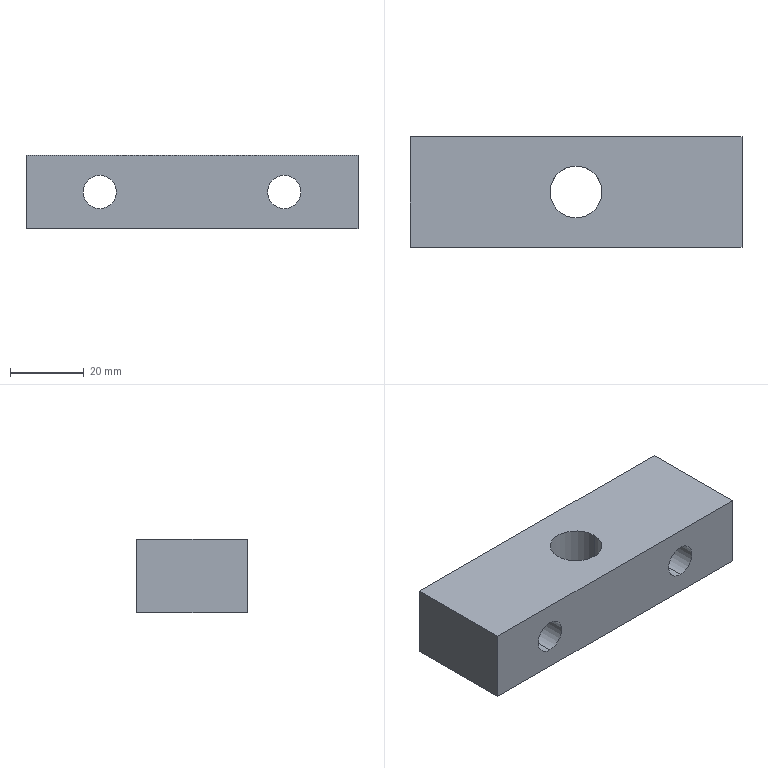Part | STEP file | M-05-2507_default | 1 solid | 18 faces | box 90 x 30 x 20 mm | volume 45159 mm3 | cylinder 10 | plane 8 | commonest cylinder face diameters 9 x4 15 x4 14 x2
STEP:
#1=CARTESIAN_POINT('',(0.,0.,0.));
#2=DIRECTION('',(0.,0.,1.));
#3=DIRECTION('',(1.,0.,0.));
#4=AXIS2_PLACEMENT_3D('',#1,#2,#3);
#5=CARTESIAN_POINT('',(38.,15.,20.));
#6=VERTEX_POINT('',#5);
#7=CARTESIAN_POINT('',(38.,15.,0.));
#8=VERTEX_POINT('',#7);
#9=CARTESIAN_POINT('',(38.,15.,0.));
#10=DIRECTION('',(0.,0.,-1.));
#11=VECTOR('',#10,1.);
#12=LINE('',#9,#11);
#13=CARTESIAN_POINT('',(45.,15.,0.));
#14=DIRECTION('',(0.,0.,-1.));
#15=DIRECTION('',(-1.,0.,0.));
#16=AXIS2_PLACEMENT_3D('',#13,#14,#15);
#17=CYLINDRICAL_SURFACE('',#16,7.);
#18=CARTESIAN_POINT('',(6.283,0.));
#19=DIRECTION('',(0.,1.));
#20=VECTOR('',#19,1.);
#21=LINE('',#18,#20);
#22=(GEOMETRIC_REPRESENTATION_CONTEXT(2)PARAMETRIC_REPRESENTATION_CONTEXT()REPRESENTATION_CONTEXT('',''));
#23=DEFINITIONAL_REPRESENTATION('',(#21),#22);
#24=PCURVE('',#17,#23);
#25=CARTESIAN_POINT('',(45.,15.,0.));
#26=DIRECTION('',(0.,0.,-1.));
#27=DIRECTION('',(-1.,0.,0.));
#28=AXIS2_PLACEMENT_3D('',#25,#26,#27);
#29=CYLINDRICAL_SURFACE('',#28,7.);
#30=CARTESIAN_POINT('',(0.,0.));
#31=DIRECTION('',(0.,1.));
#32=VECTOR('',#31,1.);
#33=LINE('',#30,#32);
#34=(GEOMETRIC_REPRESENTATION_CONTEXT(2)PARAMETRIC_REPRESENTATION_CONTEXT()REPRESENTATION_CONTEXT('',''));
#35=DEFINITIONAL_REPRESENTATION('',(#33),#34);
#36=PCURVE('',#29,#35);
#37=SURFACE_CURVE('',#12,(#24,#36),.PCURVE_S1.);
#38=EDGE_CURVE('',#6,#8,#37,.T.);
#39=ORIENTED_EDGE('',*,*,#38,.T.);
#40=CARTESIAN_POINT('',(52.,15.,0.));
#41=VERTEX_POINT('',#40);
#42=CARTESIAN_POINT('',(45.,15.,0.));
#43=DIRECTION('',(0.,0.,-1.));
#44=DIRECTION('',(-1.,0.,0.));
#45=AXIS2_PLACEMENT_3D('',#42,#43,#44);
#46=CIRCLE('',#45,7.);
#47=CARTESIAN_POINT('',(0.,0.));
#48=DIRECTION('',(1.,0.));
#49=VECTOR('',#48,1.);
#50=LINE('',#47,#49);
#51=(GEOMETRIC_REPRESENTATION_CONTEXT(2)PARAMETRIC_REPRESENTATION_CONTEXT()REPRESENTATION_CONTEXT('',''));
#52=DEFINITIONAL_REPRESENTATION('',(#50),#51);
#53=PCURVE('',#17,#52);
#54=CARTESIAN_POINT('',(0.,30.,0.));
#55=DIRECTION('',(0.,0.,-1.));
#56=DIRECTION('',(-1.,0.,0.));
#57=AXIS2_PLACEMENT_3D('',#54,#55,#56);
#58=PLANE('',#57);
#59=CARTESIAN_POINT('',(-45.,-15.));
#60=DIRECTION('',(1.,0.));
#61=AXIS2_PLACEMENT_2D('',#59,#60);
#62=CIRCLE('',#61,7.);
#63=(GEOMETRIC_REPRESENTATION_CONTEXT(2)PARAMETRIC_REPRESENTATION_CONTEXT()REPRESENTATION_CONTEXT('',''));
#64=DEFINITIONAL_REPRESENTATION('',(#62),#63);
#65=PCURVE('',#58,#64);
#66=SURFACE_CURVE('',#46,(#53,#65),.PCURVE_S1.);
#67=EDGE_CURVE('',#41,#8,#66,.T.);
#68=ORIENTED_EDGE('',*,*,#67,.F.);
#69=CARTESIAN_POINT('',(52.,15.,20.));
#70=VERTEX_POINT('',#69);
#71=CARTESIAN_POINT('',(52.,15.,0.));
#72=DIRECTION('',(0.,0.,-1.));
#73=VECTOR('',#72,1.);
#74=LINE('',#71,#73);
#75=CARTESIAN_POINT('',(3.142,0.));
#76=DIRECTION('',(0.,1.));
#77=VECTOR('',#76,1.);
#78=LINE('',#75,#77);
#79=(GEOMETRIC_REPRESENTATION_CONTEXT(2)PARAMETRIC_REPRESENTATION_CONTEXT()REPRESENTATION_CONTEXT('',''));
#80=DEFINITIONAL_REPRESENTATION('',(#78),#79);
#81=PCURVE('',#17,#80);
#82=CARTESIAN_POINT('',(3.142,0.));
#83=DIRECTION('',(0.,1.));
#84=VECTOR('',#83,1.);
#85=LINE('',#82,#84);
#86=(GEOMETRIC_REPRESENTATION_CONTEXT(2)PARAMETRIC_REPRESENTATION_CONTEXT()REPRESENTATION_CONTEXT('',''));
#87=DEFINITIONAL_REPRESENTATION('',(#85),#86);
#88=PCURVE('',#29,#87);
#89=SURFACE_CURVE('',#74,(#81,#88),.PCURVE_S1.);
#90=EDGE_CURVE('',#70,#41,#89,.T.);
#91=ORIENTED_EDGE('',*,*,#90,.F.);
#92=CARTESIAN_POINT('',(45.,15.,20.));
#93=DIRECTION('',(0.,0.,-1.));
#94=DIRECTION('',(-1.,0.,0.));
#95=AXIS2_PLACEMENT_3D('',#92,#93,#94);
#96=CIRCLE('',#95,7.);
#97=CARTESIAN_POINT('',(0.,-20.));
#98=DIRECTION('',(1.,0.));
#99=VECTOR('',#98,1.);
#100=LINE('',#97,#99);
#101=(GEOMETRIC_REPRESENTATION_CONTEXT(2)PARAMETRIC_REPRESENTATION_CONTEXT()REPRESENTATION_CONTEXT('',''));
#102=DEFINITIONAL_REPRESENTATION('',(#100),#101);
#103=PCURVE('',#17,#102);
#104=CARTESIAN_POINT('',(0.,30.,20.));
#105=DIRECTION('',(0.,0.,-1.));
#106=DIRECTION('',(-1.,0.,0.));
#107=AXIS2_PLACEMENT_3D('',#104,#105,#106);
#108=PLANE('',#107);
#109=CARTESIAN_POINT('',(-45.,-15.));
#110=DIRECTION('',(1.,0.));
#111=AXIS2_PLACEMENT_2D('',#109,#110);
#112=CIRCLE('',#111,7.);
#113=(GEOMETRIC_REPRESENTATION_CONTEXT(2)PARAMETRIC_REPRESENTATION_CONTEXT()REPRESENTATION_CONTEXT('',''));
#114=DEFINITIONAL_REPRESENTATION('',(#112),#113);
#115=PCURVE('',#108,#114);
#116=SURFACE_CURVE('',#96,(#103,#115),.PCURVE_S1.);
#117=EDGE_CURVE('',#70,#6,#116,.T.);
#118=ORIENTED_EDGE('',*,*,#117,.T.);
#119=EDGE_LOOP('',(#39,#68,#91,#118));
#120=FACE_BOUND('',#119,.F.);
#121=ADVANCED_FACE('',(#120),#17,.F.);
#122=CARTESIAN_POINT('',(20.,21.4,17.5));
#123=VERTEX_POINT('',#122);
#124=CARTESIAN_POINT('',(20.,30.,17.5));
#125=VERTEX_POINT('',#124);
#126=CARTESIAN_POINT('',(20.,30.,17.5));
#127=DIRECTION('',(0.,1.,0.));
#128=VECTOR('',#127,1.);
#129=LINE('',#126,#128);
#130=CARTESIAN_POINT('',(20.,30.,10.));
#131=DIRECTION('',(0.,1.,0.));
#132=DIRECTION('',(0.,0.,1.));
#133=AXIS2_PLACEMENT_3D('',#130,#131,#132);
#134=CYLINDRICAL_SURFACE('',#133,7.5);
#135=CARTESIAN_POINT('',(6.283,0.));
#136=DIRECTION('',(0.,1.));
#137=VECTOR('',#136,1.);
#138=LINE('',#135,#137);
#139=(GEOMETRIC_REPRESENTATION_CONTEXT(2)PARAMETRIC_REPRESENTATION_CONTEXT()REPRESENTATION_CONTEXT('',''));
#140=DEFINITIONAL_REPRESENTATION('',(#138),#139);
#141=PCURVE('',#134,#140);
#142=CARTESIAN_POINT('',(20.,30.,10.));
#143=DIRECTION('',(0.,1.,0.));
#144=DIRECTION('',(0.,0.,1.));
#145=AXIS2_PLACEMENT_3D('',#142,#143,#144);
#146=CYLINDRICAL_SURFACE('',#145,7.5);
#147=CARTESIAN_POINT('',(0.,0.));
#148=DIRECTION('',(0.,1.));
#149=VECTOR('',#148,1.);
#150=LINE('',#147,#149);
#151=(GEOMETRIC_REPRESENTATION_CONTEXT(2)PARAMETRIC_REPRESENTATION_CONTEXT()REPRESENTATION_CONTEXT('',''));
#152=DEFINITIONAL_REPRESENTATION('',(#150),#151);
#153=PCURVE('',#146,#152);
#154=SURFACE_CURVE('',#129,(#141,#153),.PCURVE_S1.);
#155=EDGE_CURVE('',#123,#125,#154,.T.);
#156=ORIENTED_EDGE('',*,*,#155,.T.);
#157=CARTESIAN_POINT('',(20.,30.,2.5));
#158=VERTEX_POINT('',#157);
#159=CARTESIAN_POINT('',(20.,30.,10.));
#160=DIRECTION('',(0.,1.,0.));
#161=DIRECTION('',(0.,0.,1.));
#162=AXIS2_PLACEMENT_3D('',#159,#160,#161);
#163=CIRCLE('',#162,7.5);
#164=CARTESIAN_POINT('',(0.,0.));
#165=DIRECTION('',(1.,0.));
#166=VECTOR('',#165,1.);
#167=LINE('',#164,#166);
#168=(GEOMETRIC_REPRESENTATION_CONTEXT(2)PARAMETRIC_REPRESENTATION_CONTEXT()REPRESENTATION_CONTEXT('',''));
#169=DEFINITIONAL_REPRESENTATION('',(#167),#168);
#170=PCURVE('',#134,#169);
#171=CARTESIAN_POINT('',(0.,30.,20.));
#172=DIRECTION('',(0.,-1.,0.));
#173=DIRECTION('',(0.,0.,-1.));
#174=AXIS2_PLACEMENT_3D('',#171,#172,#173);
#175=PLANE('',#174);
#176=CARTESIAN_POINT('',(2.5,20.));
#177=CARTESIAN_POINT('',(2.5,32.99));
#178=CARTESIAN_POINT('',(13.75,26.495));
#179=CARTESIAN_POINT('',(25.,20.));
#180=CARTESIAN_POINT('',(13.75,13.505));
#181=CARTESIAN_POINT('',(2.5,7.01));
#182=CARTESIAN_POINT('',(2.5,20.));
#183=(BOUNDED_CURVE()B_SPLINE_CURVE(2,(#176,#177,#178,#179,#180,#181,#182),.UNSPECIFIED.,.T.,.F.)B_SPLINE_CURVE_WITH_KNOTS((1,2,2,2,2,1),(-2.094,0.,2.094,4.189,6.283,8.378),.UNSPECIFIED.)CURVE()GEOMETRIC_REPRESENTATION_ITEM()RATIONAL_B_SPLINE_CURVE((1.,0.5,1.,0.5,1.,0.5,1.))REPRESENTATION_ITEM(''));
#184=(GEOMETRIC_REPRESENTATION_CONTEXT(2)PARAMETRIC_REPRESENTATION_CONTEXT()REPRESENTATION_CONTEXT('',''));
#185=DEFINITIONAL_REPRESENTATION('',(#183),#184);
#186=PCURVE('',#175,#185);
#187=SURFACE_CURVE('',#163,(#170,#186),.PCURVE_S1.);
#188=EDGE_CURVE('',#158,#125,#187,.T.);
#189=ORIENTED_EDGE('',*,*,#188,.F.);
#190=CARTESIAN_POINT('',(20.,21.4,2.5));
#191=VERTEX_POINT('',#190);
#192=CARTESIAN_POINT('',(20.,30.,2.5));
#193=DIRECTION('',(0.,1.,0.));
#194=VECTOR('',#193,1.);
#195=LINE('',#192,#194);
#196=CARTESIAN_POINT('',(3.142,0.));
#197=DIRECTION('',(0.,1.));
#198=VECTOR('',#197,1.);
#199=LINE('',#196,#198);
#200=(GEOMETRIC_REPRESENTATION_CONTEXT(2)PARAMETRIC_REPRESENTATION_CONTEXT()REPRESENTATION_CONTEXT('',''));
#201=DEFINITIONAL_REPRESENTATION('',(#199),#200);
#202=PCURVE('',#134,#201);
#203=CARTESIAN_POINT('',(3.142,0.));
#204=DIRECTION('',(0.,1.));
#205=VECTOR('',#204,1.);
#206=LINE('',#203,#205);
#207=(GEOMETRIC_REPRESENTATION_CONTEXT(2)PARAMETRIC_REPRESENTATION_CONTEXT()REPRESENTATION_CONTEXT('',''));
#208=DEFINITIONAL_REPRESENTATION('',(#206),#207);
#209=PCURVE('',#146,#208);
#210=SURFACE_CURVE('',#195,(#202,#209),.PCURVE_S1.);
#211=EDGE_CURVE('',#191,#158,#210,.T.);
#212=ORIENTED_EDGE('',*,*,#211,.F.);
#213=CARTESIAN_POINT('',(20.,21.4,10.));
#214=DIRECTION('',(0.,1.,0.));
#215=DIRECTION('',(0.,0.,1.));
#216=AXIS2_PLACEMENT_3D('',#213,#214,#215);
#217=CIRCLE('',#216,7.5);
#218=CARTESIAN_POINT('',(0.,-8.6));
#219=DIRECTION('',(1.,0.));
#220=VECTOR('',#219,1.);
#221=LINE('',#218,#220);
#222=(GEOMETRIC_REPRESENTATION_CONTEXT(2)PARAMETRIC_REPRESENTATION_CONTEXT()REPRESENTATION_CONTEXT('',''));
#223=DEFINITIONAL_REPRESENTATION('',(#221),#222);
#224=PCURVE('',#134,#223);
#225=CARTESIAN_POINT('',(24.5,21.4,10.));
#226=DIRECTION('',(0.,-1.,0.));
#227=DIRECTION('',(0.,0.,-1.));
#228=AXIS2_PLACEMENT_3D('',#225,#226,#227);
#229=PLANE('',#228);
#230=CARTESIAN_POINT('',(-7.5,-4.5));
#231=CARTESIAN_POINT('',(-7.5,8.49));
#232=CARTESIAN_POINT('',(3.75,1.995));
#233=CARTESIAN_POINT('',(15.,-4.5));
#234=CARTESIAN_POINT('',(3.75,-10.995));
#235=CARTESIAN_POINT('',(-7.5,-17.49));
#236=CARTESIAN_POINT('',(-7.5,-4.5));
#237=(BOUNDED_CURVE()B_SPLINE_CURVE(2,(#230,#231,#232,#233,#234,#235,#236),.UNSPECIFIED.,.T.,.F.)B_SPLINE_CURVE_WITH_KNOTS((1,2,2,2,2,1),(-2.094,0.,2.094,4.189,6.283,8.378),.UNSPECIFIED.)CURVE()GEOMETRIC_REPRESENTATION_ITEM()RATIONAL_B_SPLINE_CURVE((1.,0.5,1.,0.5,1.,0.5,1.))REPRESENTATION_ITEM(''));
#238=(GEOMETRIC_REPRESENTATION_CONTEXT(2)PARAMETRIC_REPRESENTATION_CONTEXT()REPRESENTATION_CONTEXT('',''));
#239=DEFINITIONAL_REPRESENTATION('',(#237),#238);
#240=PCURVE('',#229,#239);
#241=SURFACE_CURVE('',#217,(#224,#240),.PCURVE_S1.);
#242=EDGE_CURVE('',#191,#123,#241,.T.);
#243=ORIENTED_EDGE('',*,*,#242,.T.);
#244=EDGE_LOOP('',(#156,#189,#212,#243));
#245=FACE_BOUND('',#244,.F.);
#246=ADVANCED_FACE('',(#245),#134,.F.);
#247=CARTESIAN_POINT('',(20.,0.,14.5));
#248=VERTEX_POINT('',#247);
#249=CARTESIAN_POINT('',(20.,21.4,14.5));
#250=VERTEX_POINT('',#249);
#251=CARTESIAN_POINT('',(20.,30.,14.5));
#252=DIRECTION('',(0.,1.,0.));
#253=VECTOR('',#252,1.);
#254=LINE('',#251,#253);
#255=CARTESIAN_POINT('',(20.,30.,10.));
#256=DIRECTION('',(0.,1.,0.));
#257=DIRECTION('',(0.,0.,1.));
#258=AXIS2_PLACEMENT_3D('',#255,#256,#257);
#259=CYLINDRICAL_SURFACE('',#258,4.5);
#260=CARTESIAN_POINT('',(6.283,0.));
#261=DIRECTION('',(0.,1.));
#262=VECTOR('',#261,1.);
#263=LINE('',#260,#262);
#264=(GEOMETRIC_REPRESENTATION_CONTEXT(2)PARAMETRIC_REPRESENTATION_CONTEXT()REPRESENTATION_CONTEXT('',''));
#265=DEFINITIONAL_REPRESENTATION('',(#263),#264);
#266=PCURVE('',#259,#265);
#267=CARTESIAN_POINT('',(20.,30.,10.));
#268=DIRECTION('',(0.,1.,0.));
#269=DIRECTION('',(0.,0.,1.));
#270=AXIS2_PLACEMENT_3D('',#267,#268,#269);
#271=CYLINDRICAL_SURFACE('',#270,4.5);
#272=CARTESIAN_POINT('',(0.,0.));
#273=DIRECTION('',(0.,1.));
#274=VECTOR('',#273,1.);
#275=LINE('',#272,#274);
#276=(GEOMETRIC_REPRESENTATION_CONTEXT(2)PARAMETRIC_REPRESENTATION_CONTEXT()REPRESENTATION_CONTEXT('',''));
#277=DEFINITIONAL_REPRESENTATION('',(#275),#276);
#278=PCURVE('',#271,#277);
#279=SURFACE_CURVE('',#254,(#266,#278),.PCURVE_S1.);
#280=EDGE_CURVE('',#248,#250,#279,.T.);
#281=ORIENTED_EDGE('',*,*,#280,.T.);
#282=CARTESIAN_POINT('',(20.,21.4,5.5));
#283=VERTEX_POINT('',#282);
#284=CARTESIAN_POINT('',(20.,21.4,10.));
#285=DIRECTION('',(0.,1.,0.));
#286=DIRECTION('',(0.,0.,1.));
#287=AXIS2_PLACEMENT_3D('',#284,#285,#286);
#288=CIRCLE('',#287,4.5);
#289=CARTESIAN_POINT('',(0.,-8.6));
#290=DIRECTION('',(1.,0.));
#291=VECTOR('',#290,1.);
#292=LINE('',#289,#291);
#293=(GEOMETRIC_REPRESENTATION_CONTEXT(2)PARAMETRIC_REPRESENTATION_CONTEXT()REPRESENTATION_CONTEXT('',''));
#294=DEFINITIONAL_REPRESENTATION('',(#292),#293);
#295=PCURVE('',#259,#294);
#296=CARTESIAN_POINT('',(-4.5,-4.5));
#297=CARTESIAN_POINT('',(-4.5,3.294));
#298=CARTESIAN_POINT('',(2.25,-0.6029));
#299=CARTESIAN_POINT('',(9.,-4.5));
#300=CARTESIAN_POINT('',(2.25,-8.397));
#301=CARTESIAN_POINT('',(-4.5,-12.294));
#302=CARTESIAN_POINT('',(-4.5,-4.5));
#303=(BOUNDED_CURVE()B_SPLINE_CURVE(2,(#296,#297,#298,#299,#300,#301,#302),.UNSPECIFIED.,.T.,.F.)B_SPLINE_CURVE_WITH_KNOTS((1,2,2,2,2,1),(-2.094,0.,2.094,4.189,6.283,8.378),.UNSPECIFIED.)CURVE()GEOMETRIC_REPRESENTATION_ITEM()RATIONAL_B_SPLINE_CURVE((1.,0.5,1.,0.5,1.,0.5,1.))REPRESENTATION_ITEM(''));
#304=(GEOMETRIC_REPRESENTATION_CONTEXT(2)PARAMETRIC_REPRESENTATION_CONTEXT()REPRESENTATION_CONTEXT('',''));
#305=DEFINITIONAL_REPRESENTATION('',(#303),#304);
#306=PCURVE('',#229,#305);
#307=SURFACE_CURVE('',#288,(#295,#306),.PCURVE_S1.);
#308=EDGE_CURVE('',#283,#250,#307,.T.);
#309=ORIENTED_EDGE('',*,*,#308,.F.);
#310=CARTESIAN_POINT('',(20.,0.,5.5));
#311=VERTEX_POINT('',#310);
#312=CARTESIAN_POINT('',(20.,30.,5.5));
#313=DIRECTION('',(0.,1.,0.));
#314=VECTOR('',#313,1.);
#315=LINE('',#312,#314);
#316=CARTESIAN_POINT('',(3.142,0.));
#317=DIRECTION('',(0.,1.));
#318=VECTOR('',#317,1.);
#319=LINE('',#316,#318);
#320=(GEOMETRIC_REPRESENTATION_CONTEXT(2)PARAMETRIC_REPRESENTATION_CONTEXT()REPRESENTATION_CONTEXT('',''));
#321=DEFINITIONAL_REPRESENTATION('',(#319),#320);
#322=PCURVE('',#259,#321);
#323=CARTESIAN_POINT('',(3.142,0.));
#324=DIRECTION('',(0.,1.));
#325=VECTOR('',#324,1.);
#326=LINE('',#323,#325);
#327=(GEOMETRIC_REPRESENTATION_CONTEXT(2)PARAMETRIC_REPRESENTATION_CONTEXT()REPRESENTATION_CONTEXT('',''));
#328=DEFINITIONAL_REPRESENTATION('',(#326),#327);
#329=PCURVE('',#271,#328);
#330=SURFACE_CURVE('',#315,(#322,#329),.PCURVE_S1.);
#331=EDGE_CURVE('',#311,#283,#330,.T.);
#332=ORIENTED_EDGE('',*,*,#331,.F.);
#333=CARTESIAN_POINT('',(20.,0.,10.));
#334=DIRECTION('',(0.,1.,0.));
#335=DIRECTION('',(0.,0.,1.));
#336=AXIS2_PLACEMENT_3D('',#333,#334,#335);
#337=CIRCLE('',#336,4.5);
#338=CARTESIAN_POINT('',(0.,-30.));
#339=DIRECTION('',(1.,0.));
#340=VECTOR('',#339,1.);
#341=LINE('',#338,#340);
#342=(GEOMETRIC_REPRESENTATION_CONTEXT(2)PARAMETRIC_REPRESENTATION_CONTEXT()REPRESENTATION_CONTEXT('',''));
#343=DEFINITIONAL_REPRESENTATION('',(#341),#342);
#344=PCURVE('',#259,#343);
#345=CARTESIAN_POINT('',(0.,0.,20.));
#346=DIRECTION('',(0.,1.,0.));
#347=DIRECTION('',(0.,0.,1.));
#348=AXIS2_PLACEMENT_3D('',#345,#346,#347);
#349=PLANE('',#348);
#350=CARTESIAN_POINT('',(-10.,20.));
#351=DIRECTION('',(1.,0.));
#352=AXIS2_PLACEMENT_2D('',#350,#351);
#353=CIRCLE('',#352,4.5);
#354=(GEOMETRIC_REPRESENTATION_CONTEXT(2)PARAMETRIC_REPRESENTATION_CONTEXT()REPRESENTATION_CONTEXT('',''));
#355=DEFINITIONAL_REPRESENTATION('',(#353),#354);
#356=PCURVE('',#349,#355);
#357=SURFACE_CURVE('',#337,(#344,#356),.PCURVE_S1.);
#358=EDGE_CURVE('',#311,#248,#357,.T.);
#359=ORIENTED_EDGE('',*,*,#358,.T.);
#360=EDGE_LOOP('',(#281,#309,#332,#359));
#361=FACE_BOUND('',#360,.F.);
#362=ADVANCED_FACE('',(#361),#259,.F.);
#363=CARTESIAN_POINT('',(70.,21.4,17.5));
#364=VERTEX_POINT('',#363);
#365=CARTESIAN_POINT('',(70.,30.,17.5));
#366=VERTEX_POINT('',#365);
#367=CARTESIAN_POINT('',(70.,30.,17.5));
#368=DIRECTION('',(0.,1.,0.));
#369=VECTOR('',#368,1.);
#370=LINE('',#367,#369);
#371=CARTESIAN_POINT('',(70.,30.,10.));
#372=DIRECTION('',(0.,1.,0.));
#373=DIRECTION('',(0.,0.,1.));
#374=AXIS2_PLACEMENT_3D('',#371,#372,#373);
#375=CYLINDRICAL_SURFACE('',#374,7.5);
#376=CARTESIAN_POINT('',(6.283,0.));
#377=DIRECTION('',(0.,1.));
#378=VECTOR('',#377,1.);
#379=LINE('',#376,#378);
#380=(GEOMETRIC_REPRESENTATION_CONTEXT(2)PARAMETRIC_REPRESENTATION_CONTEXT()REPRESENTATION_CONTEXT('',''));
#381=DEFINITIONAL_REPRESENTATION('',(#379),#380);
#382=PCURVE('',#375,#381);
#383=CARTESIAN_POINT('',(70.,30.,10.));
#384=DIRECTION('',(0.,1.,0.));
#385=DIRECTION('',(0.,0.,1.));
#386=AXIS2_PLACEMENT_3D('',#383,#384,#385);
#387=CYLINDRICAL_SURFACE('',#386,7.5);
#388=CARTESIAN_POINT('',(0.,0.));
#389=DIRECTION('',(0.,1.));
#390=VECTOR('',#389,1.);
#391=LINE('',#388,#390);
#392=(GEOMETRIC_REPRESENTATION_CONTEXT(2)PARAMETRIC_REPRESENTATION_CONTEXT()REPRESENTATION_CONTEXT('',''));
#393=DEFINITIONAL_REPRESENTATION('',(#391),#392);
#394=PCURVE('',#387,#393);
#395=SURFACE_CURVE('',#370,(#382,#394),.PCURVE_S1.);
#396=EDGE_CURVE('',#364,#366,#395,.T.);
#397=ORIENTED_EDGE('',*,*,#396,.T.);
#398=CARTESIAN_POINT('',(70.,30.,2.5));
#399=VERTEX_POINT('',#398);
#400=CARTESIAN_POINT('',(70.,30.,10.));
#401=DIRECTION('',(0.,1.,0.));
#402=DIRECTION('',(0.,0.,1.));
#403=AXIS2_PLACEMENT_3D('',#400,#401,#402);
#404=CIRCLE('',#403,7.5);
#405=CARTESIAN_POINT('',(0.,0.));
#406=DIRECTION('',(1.,0.));
#407=VECTOR('',#406,1.);
#408=LINE('',#405,#407);
#409=(GEOMETRIC_REPRESENTATION_CONTEXT(2)PARAMETRIC_REPRESENTATION_CONTEXT()REPRESENTATION_CONTEXT('',''));
#410=DEFINITIONAL_REPRESENTATION('',(#408),#409);
#411=PCURVE('',#375,#410);
#412=CARTESIAN_POINT('',(2.5,70.));
#413=CARTESIAN_POINT('',(2.5,82.99));
#414=CARTESIAN_POINT('',(13.75,76.495));
#415=CARTESIAN_POINT('',(25.,70.));
#416=CARTESIAN_POINT('',(13.75,63.505));
#417=CARTESIAN_POINT('',(2.5,57.01));
#418=CARTESIAN_POINT('',(2.5,70.));
#419=(BOUNDED_CURVE()B_SPLINE_CURVE(2,(#412,#413,#414,#415,#416,#417,#418),.UNSPECIFIED.,.T.,.F.)B_SPLINE_CURVE_WITH_KNOTS((1,2,2,2,2,1),(-2.094,0.,2.094,4.189,6.283,8.378),.UNSPECIFIED.)CURVE()GEOMETRIC_REPRESENTATION_ITEM()RATIONAL_B_SPLINE_CURVE((1.,0.5,1.,0.5,1.,0.5,1.))REPRESENTATION_ITEM(''));
#420=(GEOMETRIC_REPRESENTATION_CONTEXT(2)PARAMETRIC_REPRESENTATION_CONTEXT()REPRESENTATION_CONTEXT('',''));
#421=DEFINITIONAL_REPRESENTATION('',(#419),#420);
#422=PCURVE('',#175,#421);
#423=SURFACE_CURVE('',#404,(#411,#422),.PCURVE_S1.);
#424=EDGE_CURVE('',#399,#366,#423,.T.);
#425=ORIENTED_EDGE('',*,*,#424,.F.);
#426=CARTESIAN_POINT('',(70.,21.4,2.5));
#427=VERTEX_POINT('',#426);
#428=CARTESIAN_POINT('',(70.,30.,2.5));
#429=DIRECTION('',(0.,1.,0.));
#430=VECTOR('',#429,1.);
#431=LINE('',#428,#430);
#432=CARTESIAN_POINT('',(3.142,0.));
#433=DIRECTION('',(0.,1.));
#434=VECTOR('',#433,1.);
#435=LINE('',#432,#434);
#436=(GEOMETRIC_REPRESENTATION_CONTEXT(2)PARAMETRIC_REPRESENTATION_CONTEXT()REPRESENTATION_CONTEXT('',''));
#437=DEFINITIONAL_REPRESENTATION('',(#435),#436);
#438=PCURVE('',#375,#437);
#439=CARTESIAN_POINT('',(3.142,0.));
#440=DIRECTION('',(0.,1.));
#441=VECTOR('',#440,1.);
#442=LINE('',#439,#441);
#443=(GEOMETRIC_REPRESENTATION_CONTEXT(2)PARAMETRIC_REPRESENTATION_CONTEXT()REPRESENTATION_CONTEXT('',''));
#444=DEFINITIONAL_REPRESENTATION('',(#442),#443);
#445=PCURVE('',#387,#444);
#446=SURFACE_CURVE('',#431,(#438,#445),.PCURVE_S1.);
#447=EDGE_CURVE('',#427,#399,#446,.T.);
#448=ORIENTED_EDGE('',*,*,#447,.F.);
#449=CARTESIAN_POINT('',(70.,21.4,10.));
#450=DIRECTION('',(0.,1.,0.));
#451=DIRECTION('',(0.,0.,1.));
#452=AXIS2_PLACEMENT_3D('',#449,#450,#451);
#453=CIRCLE('',#452,7.5);
#454=CARTESIAN_POINT('',(0.,-8.6));
#455=DIRECTION('',(1.,0.));
#456=VECTOR('',#455,1.);
#457=LINE('',#454,#456);
#458=(GEOMETRIC_REPRESENTATION_CONTEXT(2)PARAMETRIC_REPRESENTATION_CONTEXT()REPRESENTATION_CONTEXT('',''));
#459=DEFINITIONAL_REPRESENTATION('',(#457),#458);
#460=PCURVE('',#375,#459);
#461=CARTESIAN_POINT('',(74.5,21.4,10.));
#462=DIRECTION('',(0.,-1.,0.));
#463=DIRECTION('',(0.,0.,-1.));
#464=AXIS2_PLACEMENT_3D('',#461,#462,#463);
#465=PLANE('',#464);
#466=CARTESIAN_POINT('',(-7.5,-4.5));
#467=CARTESIAN_POINT('',(-7.5,8.49));
#468=CARTESIAN_POINT('',(3.75,1.995));
#469=CARTESIAN_POINT('',(15.,-4.5));
#470=CARTESIAN_POINT('',(3.75,-10.995));
#471=CARTESIAN_POINT('',(-7.5,-17.49));
#472=CARTESIAN_POINT('',(-7.5,-4.5));
#473=(BOUNDED_CURVE()B_SPLINE_CURVE(2,(#466,#467,#468,#469,#470,#471,#472),.UNSPECIFIED.,.T.,.F.)B_SPLINE_CURVE_WITH_KNOTS((1,2,2,2,2,1),(-2.094,0.,2.094,4.189,6.283,8.378),.UNSPECIFIED.)CURVE()GEOMETRIC_REPRESENTATION_ITEM()RATIONAL_B_SPLINE_CURVE((1.,0.5,1.,0.5,1.,0.5,1.))REPRESENTATION_ITEM(''));
#474=(GEOMETRIC_REPRESENTATION_CONTEXT(2)PARAMETRIC_REPRESENTATION_CONTEXT()REPRESENTATION_CONTEXT('',''));
#475=DEFINITIONAL_REPRESENTATION('',(#473),#474);
#476=PCURVE('',#465,#475);
#477=SURFACE_CURVE('',#453,(#460,#476),.PCURVE_S1.);
#478=EDGE_CURVE('',#427,#364,#477,.T.);
#479=ORIENTED_EDGE('',*,*,#478,.T.);
#480=EDGE_LOOP('',(#397,#425,#448,#479));
#481=FACE_BOUND('',#480,.F.);
#482=ADVANCED_FACE('',(#481),#375,.F.);
#483=CARTESIAN_POINT('',(70.,0.,14.5));
#484=VERTEX_POINT('',#483);
#485=CARTESIAN_POINT('',(70.,21.4,14.5));
#486=VERTEX_POINT('',#485);
#487=CARTESIAN_POINT('',(70.,30.,14.5));
#488=DIRECTION('',(0.,1.,0.));
#489=VECTOR('',#488,1.);
#490=LINE('',#487,#489);
#491=CARTESIAN_POINT('',(70.,30.,10.));
#492=DIRECTION('',(0.,1.,0.));
#493=DIRECTION('',(0.,0.,1.));
#494=AXIS2_PLACEMENT_3D('',#491,#492,#493);
#495=CYLINDRICAL_SURFACE('',#494,4.5);
#496=CARTESIAN_POINT('',(6.283,0.));
#497=DIRECTION('',(0.,1.));
#498=VECTOR('',#497,1.);
#499=LINE('',#496,#498);
#500=(GEOMETRIC_REPRESENTATION_CONTEXT(2)PARAMETRIC_REPRESENTATION_CONTEXT()REPRESENTATION_CONTEXT('',''));
#501=DEFINITIONAL_REPRESENTATION('',(#499),#500);
#502=PCURVE('',#495,#501);
#503=CARTESIAN_POINT('',(70.,30.,10.));
#504=DIRECTION('',(0.,1.,0.));
#505=DIRECTION('',(0.,0.,1.));
#506=AXIS2_PLACEMENT_3D('',#503,#504,#505);
#507=CYLINDRICAL_SURFACE('',#506,4.5);
#508=CARTESIAN_POINT('',(0.,0.));
#509=DIRECTION('',(0.,1.));
#510=VECTOR('',#509,1.);
#511=LINE('',#508,#510);
#512=(GEOMETRIC_REPRESENTATION_CONTEXT(2)PARAMETRIC_REPRESENTATION_CONTEXT()REPRESENTATION_CONTEXT('',''));
#513=DEFINITIONAL_REPRESENTATION('',(#511),#512);
#514=PCURVE('',#507,#513);
#515=SURFACE_CURVE('',#490,(#502,#514),.PCURVE_S1.);
#516=EDGE_CURVE('',#484,#486,#515,.T.);
#517=ORIENTED_EDGE('',*,*,#516,.T.);
#518=CARTESIAN_POINT('',(70.,21.4,5.5));
#519=VERTEX_POINT('',#518);
#520=CARTESIAN_POINT('',(70.,21.4,10.));
#521=DIRECTION('',(0.,1.,0.));
#522=DIRECTION('',(0.,0.,1.));
#523=AXIS2_PLACEMENT_3D('',#520,#521,#522);
#524=CIRCLE('',#523,4.5);
#525=CARTESIAN_POINT('',(0.,-8.6));
#526=DIRECTION('',(1.,0.));
#527=VECTOR('',#526,1.);
#528=LINE('',#525,#527);
#529=(GEOMETRIC_REPRESENTATION_CONTEXT(2)PARAMETRIC_REPRESENTATION_CONTEXT()REPRESENTATION_CONTEXT('',''));
#530=DEFINITIONAL_REPRESENTATION('',(#528),#529);
#531=PCURVE('',#495,#530);
#532=CARTESIAN_POINT('',(-4.5,-4.5));
#533=CARTESIAN_POINT('',(-4.5,3.294));
#534=CARTESIAN_POINT('',(2.25,-0.6029));
#535=CARTESIAN_POINT('',(9.,-4.5));
#536=CARTESIAN_POINT('',(2.25,-8.397));
#537=CARTESIAN_POINT('',(-4.5,-12.294));
#538=CARTESIAN_POINT('',(-4.5,-4.5));
#539=(BOUNDED_CURVE()B_SPLINE_CURVE(2,(#532,#533,#534,#535,#536,#537,#538),.UNSPECIFIED.,.T.,.F.)B_SPLINE_CURVE_WITH_KNOTS((1,2,2,2,2,1),(-2.094,0.,2.094,4.189,6.283,8.378),.UNSPECIFIED.)CURVE()GEOMETRIC_REPRESENTATION_ITEM()RATIONAL_B_SPLINE_CURVE((1.,0.5,1.,0.5,1.,0.5,1.))REPRESENTATION_ITEM(''));
#540=(GEOMETRIC_REPRESENTATION_CONTEXT(2)PARAMETRIC_REPRESENTATION_CONTEXT()REPRESENTATION_CONTEXT('',''));
#541=DEFINITIONAL_REPRESENTATION('',(#539),#540);
#542=PCURVE('',#465,#541);
#543=SURFACE_CURVE('',#524,(#531,#542),.PCURVE_S1.);
#544=EDGE_CURVE('',#519,#486,#543,.T.);
#545=ORIENTED_EDGE('',*,*,#544,.F.);
#546=CARTESIAN_POINT('',(70.,0.,5.5));
#547=VERTEX_POINT('',#546);
#548=CARTESIAN_POINT('',(70.,30.,5.5));
#549=DIRECTION('',(0.,1.,0.));
#550=VECTOR('',#549,1.);
#551=LINE('',#548,#550);
#552=CARTESIAN_POINT('',(3.142,0.));
#553=DIRECTION('',(0.,1.));
#554=VECTOR('',#553,1.);
#555=LINE('',#552,#554);
#556=(GEOMETRIC_REPRESENTATION_CONTEXT(2)PARAMETRIC_REPRESENTATION_CONTEXT()REPRESENTATION_CONTEXT('',''));
#557=DEFINITIONAL_REPRESENTATION('',(#555),#556);
#558=PCURVE('',#495,#557);
#559=CARTESIAN_POINT('',(3.142,0.));
#560=DIRECTION('',(0.,1.));
#561=VECTOR('',#560,1.);
#562=LINE('',#559,#561);
#563=(GEOMETRIC_REPRESENTATION_CONTEXT(2)PARAMETRIC_REPRESENTATION_CONTEXT()REPRESENTATION_CONTEXT('',''));
#564=DEFINITIONAL_REPRESENTATION('',(#562),#563);
#565=PCURVE('',#507,#564);
#566=SURFACE_CURVE('',#551,(#558,#565),.PCURVE_S1.);
#567=EDGE_CURVE('',#547,#519,#566,.T.);
#568=ORIENTED_EDGE('',*,*,#567,.F.);
#569=CARTESIAN_POINT('',(70.,0.,10.));
#570=DIRECTION('',(0.,1.,0.));
#571=DIRECTION('',(0.,0.,1.));
#572=AXIS2_PLACEMENT_3D('',#569,#570,#571);
#573=CIRCLE('',#572,4.5);
#574=CARTESIAN_POINT('',(0.,-30.));
#575=DIRECTION('',(1.,0.));
#576=VECTOR('',#575,1.);
#577=LINE('',#574,#576);
#578=(GEOMETRIC_REPRESENTATION_CONTEXT(2)PARAMETRIC_REPRESENTATION_CONTEXT()REPRESENTATION_CONTEXT('',''));
#579=DEFINITIONAL_REPRESENTATION('',(#577),#578);
#580=PCURVE('',#495,#579);
#581=CARTESIAN_POINT('',(-10.,70.));
#582=DIRECTION('',(1.,0.));
#583=AXIS2_PLACEMENT_2D('',#581,#582);
#584=CIRCLE('',#583,4.5);
#585=(GEOMETRIC_REPRESENTATION_CONTEXT(2)PARAMETRIC_REPRESENTATION_CONTEXT()REPRESENTATION_CONTEXT('',''));
#586=DEFINITIONAL_REPRESENTATION('',(#584),#585);
#587=PCURVE('',#349,#586);
#588=SURFACE_CURVE('',#573,(#580,#587),.PCURVE_S1.);
#589=EDGE_CURVE('',#547,#484,#588,.T.);
#590=ORIENTED_EDGE('',*,*,#589,.T.);
#591=EDGE_LOOP('',(#517,#545,#568,#590));
#592=FACE_BOUND('',#591,.F.);
#593=ADVANCED_FACE('',(#592),#495,.F.);
#594=CARTESIAN_POINT('',(0.,30.,0.));
#595=VERTEX_POINT('',#594);
#596=CARTESIAN_POINT('',(0.,0.,0.));
#597=VERTEX_POINT('',#596);
#598=CARTESIAN_POINT('',(0.,0.,0.));
#599=DIRECTION('',(0.,-1.,0.));
#600=VECTOR('',#599,1.);
#601=LINE('',#598,#600);
#602=CARTESIAN_POINT('',(0.,0.,20.));
#603=DIRECTION('',(1.,0.,0.));
#604=DIRECTION('',(0.,0.,-1.));
#605=AXIS2_PLACEMENT_3D('',#602,#603,#604);
#606=PLANE('',#605);
#607=CARTESIAN_POINT('',(20.,0.));
#608=DIRECTION('',(0.,-1.));
#609=VECTOR('',#608,1.);
#610=LINE('',#607,#609);
#611=(GEOMETRIC_REPRESENTATION_CONTEXT(2)PARAMETRIC_REPRESENTATION_CONTEXT()REPRESENTATION_CONTEXT('',''));
#612=DEFINITIONAL_REPRESENTATION('',(#610),#611);
#613=PCURVE('',#606,#612);
#614=CARTESIAN_POINT('',(0.,-30.));
#615=DIRECTION('',(0.,-1.));
#616=VECTOR('',#615,1.);
#617=LINE('',#614,#616);
#618=(GEOMETRIC_REPRESENTATION_CONTEXT(2)PARAMETRIC_REPRESENTATION_CONTEXT()REPRESENTATION_CONTEXT('',''));
#619=DEFINITIONAL_REPRESENTATION('',(#617),#618);
#620=PCURVE('',#58,#619);
#621=SURFACE_CURVE('',#601,(#613,#620),.PCURVE_S1.);
#622=EDGE_CURVE('',#595,#597,#621,.T.);
#623=ORIENTED_EDGE('',*,*,#622,.T.);
#624=CARTESIAN_POINT('',(0.,0.,20.));
#625=VERTEX_POINT('',#624);
#626=CARTESIAN_POINT('',(0.,0.,20.));
#627=DIRECTION('',(0.,0.,-1.));
#628=VECTOR('',#627,1.);
#629=LINE('',#626,#628);
#630=CARTESIAN_POINT('',(0.,0.));
#631=DIRECTION('',(1.,0.));
#632=VECTOR('',#631,1.);
#633=LINE('',#630,#632);
#634=(GEOMETRIC_REPRESENTATION_CONTEXT(2)PARAMETRIC_REPRESENTATION_CONTEXT()REPRESENTATION_CONTEXT('',''));
#635=DEFINITIONAL_REPRESENTATION('',(#633),#634);
#636=PCURVE('',#606,#635);
#637=CARTESIAN_POINT('',(0.,0.));
#638=DIRECTION('',(-1.,0.));
#639=VECTOR('',#638,1.);
#640=LINE('',#637,#639);
#641=(GEOMETRIC_REPRESENTATION_CONTEXT(2)PARAMETRIC_REPRESENTATION_CONTEXT()REPRESENTATION_CONTEXT('',''));
#642=DEFINITIONAL_REPRESENTATION('',(#640),#641);
#643=PCURVE('',#349,#642);
#644=SURFACE_CURVE('',#629,(#636,#643),.PCURVE_S1.);
#645=EDGE_CURVE('',#625,#597,#644,.T.);
#646=ORIENTED_EDGE('',*,*,#645,.F.);
#647=CARTESIAN_POINT('',(0.,30.,20.));
#648=VERTEX_POINT('',#647);
#649=CARTESIAN_POINT('',(0.,0.,20.));
#650=DIRECTION('',(0.,-1.,0.));
#651=VECTOR('',#650,1.);
#652=LINE('',#649,#651);
#653=CARTESIAN_POINT('',(0.,0.));
#654=DIRECTION('',(0.,-1.));
#655=VECTOR('',#654,1.);
#656=LINE('',#653,#655);
#657=(GEOMETRIC_REPRESENTATION_CONTEXT(2)PARAMETRIC_REPRESENTATION_CONTEXT()REPRESENTATION_CONTEXT('',''));
#658=DEFINITIONAL_REPRESENTATION('',(#656),#657);
#659=PCURVE('',#606,#658);
#660=CARTESIAN_POINT('',(0.,-30.));
#661=DIRECTION('',(0.,-1.));
#662=VECTOR('',#661,1.);
#663=LINE('',#660,#662);
#664=(GEOMETRIC_REPRESENTATION_CONTEXT(2)PARAMETRIC_REPRESENTATION_CONTEXT()REPRESENTATION_CONTEXT('',''));
#665=DEFINITIONAL_REPRESENTATION('',(#663),#664);
#666=PCURVE('',#108,#665);
#667=SURFACE_CURVE('',#652,(#659,#666),.PCURVE_S1.);
#668=EDGE_CURVE('',#648,#625,#667,.T.);
#669=ORIENTED_EDGE('',*,*,#668,.F.);
#670=CARTESIAN_POINT('',(0.,30.,20.));
#671=DIRECTION('',(0.,0.,-1.));
#672=VECTOR('',#671,1.);
#673=LINE('',#670,#672);
#674=CARTESIAN_POINT('',(0.,30.));
#675=DIRECTION('',(1.,0.));
#676=VECTOR('',#675,1.);
#677=LINE('',#674,#676);
#678=(GEOMETRIC_REPRESENTATION_CONTEXT(2)PARAMETRIC_REPRESENTATION_CONTEXT()REPRESENTATION_CONTEXT('',''));
#679=DEFINITIONAL_REPRESENTATION('',(#677),#678);
#680=PCURVE('',#606,#679);
#681=CARTESIAN_POINT('',(0.,0.));
#682=DIRECTION('',(1.,0.));
#683=VECTOR('',#682,1.);
#684=LINE('',#681,#683);
#685=(GEOMETRIC_REPRESENTATION_CONTEXT(2)PARAMETRIC_REPRESENTATION_CONTEXT()REPRESENTATION_CONTEXT('',''));
#686=DEFINITIONAL_REPRESENTATION('',(#684),#685);
#687=PCURVE('',#175,#686);
#688=SURFACE_CURVE('',#673,(#680,#687),.PCURVE_S1.);
#689=EDGE_CURVE('',#648,#595,#688,.T.);
#690=ORIENTED_EDGE('',*,*,#689,.T.);
#691=EDGE_LOOP('',(#623,#646,#669,#690));
#692=FACE_BOUND('',#691,.T.);
#693=ADVANCED_FACE('',(#692),#606,.F.);
#694=CARTESIAN_POINT('',(20.,0.,10.));
#695=DIRECTION('',(0.,1.,0.));
#696=DIRECTION('',(0.,0.,1.));
#697=AXIS2_PLACEMENT_3D('',#694,#695,#696);
#698=CIRCLE('',#697,4.5);
#699=CARTESIAN_POINT('',(-10.,20.));
#700=DIRECTION('',(1.,0.));
#701=AXIS2_PLACEMENT_2D('',#699,#700);
#702=CIRCLE('',#701,4.5);
#703=(GEOMETRIC_REPRESENTATION_CONTEXT(2)PARAMETRIC_REPRESENTATION_CONTEXT()REPRESENTATION_CONTEXT('',''));
#704=DEFINITIONAL_REPRESENTATION('',(#702),#703);
#705=PCURVE('',#349,#704);
#706=CARTESIAN_POINT('',(0.,-30.));
#707=DIRECTION('',(1.,0.));
#708=VECTOR('',#707,1.);
#709=LINE('',#706,#708);
#710=(GEOMETRIC_REPRESENTATION_CONTEXT(2)PARAMETRIC_REPRESENTATION_CONTEXT()REPRESENTATION_CONTEXT('',''));
#711=DEFINITIONAL_REPRESENTATION('',(#709),#710);
#712=PCURVE('',#271,#711);
#713=SURFACE_CURVE('',#698,(#705,#712),.PCURVE_S1.);
#714=EDGE_CURVE('',#248,#311,#713,.T.);
#715=ORIENTED_EDGE('',*,*,#714,.T.);
#716=ORIENTED_EDGE('',*,*,#358,.T.);
#717=EDGE_LOOP('',(#715,#716));
#718=FACE_BOUND('',#717,.T.);
#719=CARTESIAN_POINT('',(70.,0.,10.));
#720=DIRECTION('',(0.,1.,0.));
#721=DIRECTION('',(0.,0.,1.));
#722=AXIS2_PLACEMENT_3D('',#719,#720,#721);
#723=CIRCLE('',#722,4.5);
#724=CARTESIAN_POINT('',(-10.,70.));
#725=DIRECTION('',(1.,0.));
#726=AXIS2_PLACEMENT_2D('',#724,#725);
#727=CIRCLE('',#726,4.5);
#728=(GEOMETRIC_REPRESENTATION_CONTEXT(2)PARAMETRIC_REPRESENTATION_CONTEXT()REPRESENTATION_CONTEXT('',''));
#729=DEFINITIONAL_REPRESENTATION('',(#727),#728);
#730=PCURVE('',#349,#729);
#731=CARTESIAN_POINT('',(0.,-30.));
#732=DIRECTION('',(1.,0.));
#733=VECTOR('',#732,1.);
#734=LINE('',#731,#733);
#735=(GEOMETRIC_REPRESENTATION_CONTEXT(2)PARAMETRIC_REPRESENTATION_CONTEXT()REPRESENTATION_CONTEXT('',''));
#736=DEFINITIONAL_REPRESENTATION('',(#734),#735);
#737=PCURVE('',#507,#736);
#738=SURFACE_CURVE('',#723,(#730,#737),.PCURVE_S1.);
#739=EDGE_CURVE('',#484,#547,#738,.T.);
#740=ORIENTED_EDGE('',*,*,#739,.T.);
#741=ORIENTED_EDGE('',*,*,#589,.T.);
#742=EDGE_LOOP('',(#740,#741));
#743=FACE_BOUND('',#742,.T.);
#744=CARTESIAN_POINT('',(90.,0.,0.));
#745=VERTEX_POINT('',#744);
#746=CARTESIAN_POINT('',(0.,0.,0.));
#747=DIRECTION('',(1.,0.,0.));
#748=VECTOR('',#747,1.);
#749=LINE('',#746,#748);
#750=CARTESIAN_POINT('',(-20.,0.));
#751=DIRECTION('',(0.,1.));
#752=VECTOR('',#751,1.);
#753=LINE('',#750,#752);
#754=(GEOMETRIC_REPRESENTATION_CONTEXT(2)PARAMETRIC_REPRESENTATION_CONTEXT()REPRESENTATION_CONTEXT('',''));
#755=DEFINITIONAL_REPRESENTATION('',(#753),#754);
#756=PCURVE('',#349,#755);
#757=CARTESIAN_POINT('',(0.,-30.));
#758=DIRECTION('',(-1.,0.));
#759=VECTOR('',#758,1.);
#760=LINE('',#757,#759);
#761=(GEOMETRIC_REPRESENTATION_CONTEXT(2)PARAMETRIC_REPRESENTATION_CONTEXT()REPRESENTATION_CONTEXT('',''));
#762=DEFINITIONAL_REPRESENTATION('',(#760),#761);
#763=PCURVE('',#58,#762);
#764=SURFACE_CURVE('',#749,(#756,#763),.PCURVE_S1.);
#765=EDGE_CURVE('',#597,#745,#764,.T.);
#766=ORIENTED_EDGE('',*,*,#765,.T.);
#767=CARTESIAN_POINT('',(90.,0.,20.));
#768=VERTEX_POINT('',#767);
#769=CARTESIAN_POINT('',(90.,0.,20.));
#770=DIRECTION('',(0.,0.,-1.));
#771=VECTOR('',#770,1.);
#772=LINE('',#769,#771);
#773=CARTESIAN_POINT('',(0.,90.));
#774=DIRECTION('',(-1.,0.));
#775=VECTOR('',#774,1.);
#776=LINE('',#773,#775);
#777=(GEOMETRIC_REPRESENTATION_CONTEXT(2)PARAMETRIC_REPRESENTATION_CONTEXT()REPRESENTATION_CONTEXT('',''));
#778=DEFINITIONAL_REPRESENTATION('',(#776),#777);
#779=PCURVE('',#349,#778);
#780=CARTESIAN_POINT('',(90.,0.,20.));
#781=DIRECTION('',(-1.,0.,0.));
#782=DIRECTION('',(0.,0.,1.));
#783=AXIS2_PLACEMENT_3D('',#780,#781,#782);
#784=PLANE('',#783);
#785=CARTESIAN_POINT('',(0.,0.));
#786=DIRECTION('',(-1.,0.));
#787=VECTOR('',#786,1.);
#788=LINE('',#785,#787);
#789=(GEOMETRIC_REPRESENTATION_CONTEXT(2)PARAMETRIC_REPRESENTATION_CONTEXT()REPRESENTATION_CONTEXT('',''));
#790=DEFINITIONAL_REPRESENTATION('',(#788),#789);
#791=PCURVE('',#784,#790);
#792=SURFACE_CURVE('',#772,(#779,#791),.PCURVE_S1.);
#793=EDGE_CURVE('',#768,#745,#792,.T.);
#794=ORIENTED_EDGE('',*,*,#793,.F.);
#795=CARTESIAN_POINT('',(0.,0.,20.));
#796=DIRECTION('',(1.,0.,0.));
#797=VECTOR('',#796,1.);
#798=LINE('',#795,#797);
#799=CARTESIAN_POINT('',(0.,0.));
#800=DIRECTION('',(0.,1.));
#801=VECTOR('',#800,1.);
#802=LINE('',#799,#801);
#803=(GEOMETRIC_REPRESENTATION_CONTEXT(2)PARAMETRIC_REPRESENTATION_CONTEXT()REPRESENTATION_CONTEXT('',''));
#804=DEFINITIONAL_REPRESENTATION('',(#802),#803);
#805=PCURVE('',#349,#804);
#806=CARTESIAN_POINT('',(0.,-30.));
#807=DIRECTION('',(-1.,0.));
#808=VECTOR('',#807,1.);
#809=LINE('',#806,#808);
#810=(GEOMETRIC_REPRESENTATION_CONTEXT(2)PARAMETRIC_REPRESENTATION_CONTEXT()REPRESENTATION_CONTEXT('',''));
#811=DEFINITIONAL_REPRESENTATION('',(#809),#810);
#812=PCURVE('',#108,#811);
#813=SURFACE_CURVE('',#798,(#805,#812),.PCURVE_S1.);
#814=EDGE_CURVE('',#625,#768,#813,.T.);
#815=ORIENTED_EDGE('',*,*,#814,.F.);
#816=ORIENTED_EDGE('',*,*,#645,.T.);
#817=EDGE_LOOP('',(#766,#794,#815,#816));
#818=FACE_BOUND('',#817,.T.);
#819=ADVANCED_FACE('',(#718,#743,#818),#349,.F.);
#820=CARTESIAN_POINT('',(90.,30.,0.));
#821=VERTEX_POINT('',#820);
#822=CARTESIAN_POINT('',(90.,0.,0.));
#823=DIRECTION('',(0.,1.,0.));
#824=VECTOR('',#823,1.);
#825=LINE('',#822,#824);
#826=CARTESIAN_POINT('',(-20.,0.));
#827=DIRECTION('',(0.,1.));
#828=VECTOR('',#827,1.);
#829=LINE('',#826,#828);
#830=(GEOMETRIC_REPRESENTATION_CONTEXT(2)PARAMETRIC_REPRESENTATION_CONTEXT()REPRESENTATION_CONTEXT('',''));
#831=DEFINITIONAL_REPRESENTATION('',(#829),#830);
#832=PCURVE('',#784,#831);
#833=CARTESIAN_POINT('',(-90.,-30.));
#834=DIRECTION('',(0.,1.));
#835=VECTOR('',#834,1.);
#836=LINE('',#833,#835);
#837=(GEOMETRIC_REPRESENTATION_CONTEXT(2)PARAMETRIC_REPRESENTATION_CONTEXT()REPRESENTATION_CONTEXT('',''));
#838=DEFINITIONAL_REPRESENTATION('',(#836),#837);
#839=PCURVE('',#58,#838);
#840=SURFACE_CURVE('',#825,(#832,#839),.PCURVE_S1.);
#841=EDGE_CURVE('',#745,#821,#840,.T.);
#842=ORIENTED_EDGE('',*,*,#841,.T.);
#843=CARTESIAN_POINT('',(90.,30.,20.));
#844=VERTEX_POINT('',#843);
#845=CARTESIAN_POINT('',(90.,30.,20.));
#846=DIRECTION('',(0.,0.,-1.));
#847=VECTOR('',#846,1.);
#848=LINE('',#845,#847);
#849=CARTESIAN_POINT('',(0.,30.));
#850=DIRECTION('',(-1.,0.));
#851=VECTOR('',#850,1.);
#852=LINE('',#849,#851);
#853=(GEOMETRIC_REPRESENTATION_CONTEXT(2)PARAMETRIC_REPRESENTATION_CONTEXT()REPRESENTATION_CONTEXT('',''));
#854=DEFINITIONAL_REPRESENTATION('',(#852),#853);
#855=PCURVE('',#784,#854);
#856=CARTESIAN_POINT('',(0.,90.));
#857=DIRECTION('',(1.,0.));
#858=VECTOR('',#857,1.);
#859=LINE('',#856,#858);
#860=(GEOMETRIC_REPRESENTATION_CONTEXT(2)PARAMETRIC_REPRESENTATION_CONTEXT()REPRESENTATION_CONTEXT('',''));
#861=DEFINITIONAL_REPRESENTATION('',(#859),#860);
#862=PCURVE('',#175,#861);
#863=SURFACE_CURVE('',#848,(#855,#862),.PCURVE_S1.);
#864=EDGE_CURVE('',#844,#821,#863,.T.);
#865=ORIENTED_EDGE('',*,*,#864,.F.);
#866=CARTESIAN_POINT('',(90.,0.,20.));
#867=DIRECTION('',(0.,1.,0.));
#868=VECTOR('',#867,1.);
#869=LINE('',#866,#868);
#870=CARTESIAN_POINT('',(0.,0.));
#871=DIRECTION('',(0.,1.));
#872=VECTOR('',#871,1.);
#873=LINE('',#870,#872);
#874=(GEOMETRIC_REPRESENTATION_CONTEXT(2)PARAMETRIC_REPRESENTATION_CONTEXT()REPRESENTATION_CONTEXT('',''));
#875=DEFINITIONAL_REPRESENTATION('',(#873),#874);
#876=PCURVE('',#784,#875);
#877=CARTESIAN_POINT('',(-90.,-30.));
#878=DIRECTION('',(0.,1.));
#879=VECTOR('',#878,1.);
#880=LINE('',#877,#879);
#881=(GEOMETRIC_REPRESENTATION_CONTEXT(2)PARAMETRIC_REPRESENTATION_CONTEXT()REPRESENTATION_CONTEXT('',''));
#882=DEFINITIONAL_REPRESENTATION('',(#880),#881);
#883=PCURVE('',#108,#882);
#884=SURFACE_CURVE('',#869,(#876,#883),.PCURVE_S1.);
#885=EDGE_CURVE('',#768,#844,#884,.T.);
#886=ORIENTED_EDGE('',*,*,#885,.F.);
#887=ORIENTED_EDGE('',*,*,#793,.T.);
#888=EDGE_LOOP('',(#842,#865,#886,#887));
#889=FACE_BOUND('',#888,.T.);
#890=ADVANCED_FACE('',(#889),#784,.F.);
#891=CARTESIAN_POINT('',(20.,30.,10.));
#892=DIRECTION('',(0.,1.,0.));
#893=DIRECTION('',(0.,0.,1.));
#894=AXIS2_PLACEMENT_3D('',#891,#892,#893);
#895=CIRCLE('',#894,7.5);
#896=CARTESIAN_POINT('',(2.5,20.));
#897=CARTESIAN_POINT('',(2.5,32.99));
#898=CARTESIAN_POINT('',(13.75,26.495));
#899=CARTESIAN_POINT('',(25.,20.));
#900=CARTESIAN_POINT('',(13.75,13.505));
#901=CARTESIAN_POINT('',(2.5,7.01));
#902=CARTESIAN_POINT('',(2.5,20.));
#903=(BOUNDED_CURVE()B_SPLINE_CURVE(2,(#896,#897,#898,#899,#900,#901,#902),.UNSPECIFIED.,.T.,.F.)B_SPLINE_CURVE_WITH_KNOTS((1,2,2,2,2,1),(-2.094,0.,2.094,4.189,6.283,8.378),.UNSPECIFIED.)CURVE()GEOMETRIC_REPRESENTATION_ITEM()RATIONAL_B_SPLINE_CURVE((1.,0.5,1.,0.5,1.,0.5,1.))REPRESENTATION_ITEM(''));
#904=(GEOMETRIC_REPRESENTATION_CONTEXT(2)PARAMETRIC_REPRESENTATION_CONTEXT()REPRESENTATION_CONTEXT('',''));
#905=DEFINITIONAL_REPRESENTATION('',(#903),#904);
#906=PCURVE('',#175,#905);
#907=CARTESIAN_POINT('',(0.,0.));
#908=DIRECTION('',(1.,0.));
#909=VECTOR('',#908,1.);
#910=LINE('',#907,#909);
#911=(GEOMETRIC_REPRESENTATION_CONTEXT(2)PARAMETRIC_REPRESENTATION_CONTEXT()REPRESENTATION_CONTEXT('',''));
#912=DEFINITIONAL_REPRESENTATION('',(#910),#911);
#913=PCURVE('',#146,#912);
#914=SURFACE_CURVE('',#895,(#906,#913),.PCURVE_S1.);
#915=EDGE_CURVE('',#125,#158,#914,.T.);
#916=ORIENTED_EDGE('',*,*,#915,.F.);
#917=ORIENTED_EDGE('',*,*,#188,.F.);
#918=EDGE_LOOP('',(#916,#917));
#919=FACE_BOUND('',#918,.T.);
#920=CARTESIAN_POINT('',(70.,30.,10.));
#921=DIRECTION('',(0.,1.,0.));
#922=DIRECTION('',(0.,0.,1.));
#923=AXIS2_PLACEMENT_3D('',#920,#921,#922);
#924=CIRCLE('',#923,7.5);
#925=CARTESIAN_POINT('',(2.5,70.));
#926=CARTESIAN_POINT('',(2.5,82.99));
#927=CARTESIAN_POINT('',(13.75,76.495));
#928=CARTESIAN_POINT('',(25.,70.));
#929=CARTESIAN_POINT('',(13.75,63.505));
#930=CARTESIAN_POINT('',(2.5,57.01));
#931=CARTESIAN_POINT('',(2.5,70.));
#932=(BOUNDED_CURVE()B_SPLINE_CURVE(2,(#925,#926,#927,#928,#929,#930,#931),.UNSPECIFIED.,.T.,.F.)B_SPLINE_CURVE_WITH_KNOTS((1,2,2,2,2,1),(-2.094,0.,2.094,4.189,6.283,8.378),.UNSPECIFIED.)CURVE()GEOMETRIC_REPRESENTATION_ITEM()RATIONAL_B_SPLINE_CURVE((1.,0.5,1.,0.5,1.,0.5,1.))REPRESENTATION_ITEM(''));
#933=(GEOMETRIC_REPRESENTATION_CONTEXT(2)PARAMETRIC_REPRESENTATION_CONTEXT()REPRESENTATION_CONTEXT('',''));
#934=DEFINITIONAL_REPRESENTATION('',(#932),#933);
#935=PCURVE('',#175,#934);
#936=CARTESIAN_POINT('',(0.,0.));
#937=DIRECTION('',(1.,0.));
#938=VECTOR('',#937,1.);
#939=LINE('',#936,#938);
#940=(GEOMETRIC_REPRESENTATION_CONTEXT(2)PARAMETRIC_REPRESENTATION_CONTEXT()REPRESENTATION_CONTEXT('',''));
#941=DEFINITIONAL_REPRESENTATION('',(#939),#940);
#942=PCURVE('',#387,#941);
#943=SURFACE_CURVE('',#924,(#935,#942),.PCURVE_S1.);
#944=EDGE_CURVE('',#366,#399,#943,.T.);
#945=ORIENTED_EDGE('',*,*,#944,.F.);
#946=ORIENTED_EDGE('',*,*,#424,.F.);
#947=EDGE_LOOP('',(#945,#946));
#948=FACE_BOUND('',#947,.T.);
#949=CARTESIAN_POINT('',(0.,30.,0.));
#950=DIRECTION('',(-1.,0.,0.));
#951=VECTOR('',#950,1.);
#952=LINE('',#949,#951);
#953=CARTESIAN_POINT('',(20.,0.));
#954=DIRECTION('',(0.,-1.));
#955=VECTOR('',#954,1.);
#956=LINE('',#953,#955);
#957=(GEOMETRIC_REPRESENTATION_CONTEXT(2)PARAMETRIC_REPRESENTATION_CONTEXT()REPRESENTATION_CONTEXT('',''));
#958=DEFINITIONAL_REPRESENTATION('',(#956),#957);
#959=PCURVE('',#175,#958);
#960=CARTESIAN_POINT('',(0.,0.));
#961=DIRECTION('',(1.,0.));
#962=VECTOR('',#961,1.);
#963=LINE('',#960,#962);
#964=(GEOMETRIC_REPRESENTATION_CONTEXT(2)PARAMETRIC_REPRESENTATION_CONTEXT()REPRESENTATION_CONTEXT('',''));
#965=DEFINITIONAL_REPRESENTATION('',(#963),#964);
#966=PCURVE('',#58,#965);
#967=SURFACE_CURVE('',#952,(#959,#966),.PCURVE_S1.);
#968=EDGE_CURVE('',#821,#595,#967,.T.);
#969=ORIENTED_EDGE('',*,*,#968,.T.);
#970=ORIENTED_EDGE('',*,*,#689,.F.);
#971=CARTESIAN_POINT('',(0.,30.,20.));
#972=DIRECTION('',(-1.,0.,0.));
#973=VECTOR('',#972,1.);
#974=LINE('',#971,#973);
#975=CARTESIAN_POINT('',(0.,0.));
#976=DIRECTION('',(0.,-1.));
#977=VECTOR('',#976,1.);
#978=LINE('',#975,#977);
#979=(GEOMETRIC_REPRESENTATION_CONTEXT(2)PARAMETRIC_REPRESENTATION_CONTEXT()REPRESENTATION_CONTEXT('',''));
#980=DEFINITIONAL_REPRESENTATION('',(#978),#979);
#981=PCURVE('',#175,#980);
#982=CARTESIAN_POINT('',(0.,0.));
#983=DIRECTION('',(1.,0.));
#984=VECTOR('',#983,1.);
#985=LINE('',#982,#984);
#986=(GEOMETRIC_REPRESENTATION_CONTEXT(2)PARAMETRIC_REPRESENTATION_CONTEXT()REPRESENTATION_CONTEXT('',''));
#987=DEFINITIONAL_REPRESENTATION('',(#985),#986);
#988=PCURVE('',#108,#987);
#989=SURFACE_CURVE('',#974,(#981,#988),.PCURVE_S1.);
#990=EDGE_CURVE('',#844,#648,#989,.T.);
#991=ORIENTED_EDGE('',*,*,#990,.F.);
#992=ORIENTED_EDGE('',*,*,#864,.T.);
#993=EDGE_LOOP('',(#969,#970,#991,#992));
#994=FACE_BOUND('',#993,.T.);
#995=ADVANCED_FACE('',(#919,#948,#994),#175,.F.);
#996=CARTESIAN_POINT('',(45.,15.,20.));
#997=DIRECTION('',(0.,0.,-1.));
#998=DIRECTION('',(-1.,0.,0.));
#999=AXIS2_PLACEMENT_3D('',#996,#997,#998);
#1000=CIRCLE('',#999,7.);
#1001=CARTESIAN_POINT('',(-45.,-15.));
#1002=DIRECTION('',(1.,0.));
#1003=AXIS2_PLACEMENT_2D('',#1001,#1002);
#1004=CIRCLE('',#1003,7.);
#1005=(GEOMETRIC_REPRESENTATION_CONTEXT(2)PARAMETRIC_REPRESENTATION_CONTEXT()REPRESENTATION_CONTEXT('',''));
#1006=DEFINITIONAL_REPRESENTATION('',(#1004),#1005);
#1007=PCURVE('',#108,#1006);
#1008=CARTESIAN_POINT('',(0.,-20.));
#1009=DIRECTION('',(1.,0.));
#1010=VECTOR('',#1009,1.);
#1011=LINE('',#1008,#1010);
#1012=(GEOMETRIC_REPRESENTATION_CONTEXT(2)PARAMETRIC_REPRESENTATION_CONTEXT()REPRESENTATION_CONTEXT('',''));
#1013=DEFINITIONAL_REPRESENTATION('',(#1011),#1012);
#1014=PCURVE('',#29,#1013);
#1015=SURFACE_CURVE('',#1000,(#1007,#1014),.PCURVE_S1.);
#1016=EDGE_CURVE('',#6,#70,#1015,.T.);
#1017=ORIENTED_EDGE('',*,*,#1016,.T.);
#1018=ORIENTED_EDGE('',*,*,#117,.T.);
#1019=EDGE_LOOP('',(#1017,#1018));
#1020=FACE_BOUND('',#1019,.T.);
#1021=ORIENTED_EDGE('',*,*,#668,.T.);
#1022=ORIENTED_EDGE('',*,*,#814,.T.);
#1023=ORIENTED_EDGE('',*,*,#885,.T.);
#1024=ORIENTED_EDGE('',*,*,#990,.T.);
#1025=EDGE_LOOP('',(#1021,#1022,#1023,#1024));
#1026=FACE_BOUND('',#1025,.T.);
#1027=ADVANCED_FACE('',(#1020,#1026),#108,.F.);
#1028=CARTESIAN_POINT('',(45.,15.,0.));
#1029=DIRECTION('',(0.,0.,-1.));
#1030=DIRECTION('',(-1.,0.,0.));
#1031=AXIS2_PLACEMENT_3D('',#1028,#1029,#1030);
#1032=CIRCLE('',#1031,7.);
#1033=CARTESIAN_POINT('',(-45.,-15.));
#1034=DIRECTION('',(1.,0.));
#1035=AXIS2_PLACEMENT_2D('',#1033,#1034);
#1036=CIRCLE('',#1035,7.);
#1037=(GEOMETRIC_REPRESENTATION_CONTEXT(2)PARAMETRIC_REPRESENTATION_CONTEXT()REPRESENTATION_CONTEXT('',''));
#1038=DEFINITIONAL_REPRESENTATION('',(#1036),#1037);
#1039=PCURVE('',#58,#1038);
#1040=CARTESIAN_POINT('',(0.,0.));
#1041=DIRECTION('',(1.,0.));
#1042=VECTOR('',#1041,1.);
#1043=LINE('',#1040,#1042);
#1044=(GEOMETRIC_REPRESENTATION_CONTEXT(2)PARAMETRIC_REPRESENTATION_CONTEXT()REPRESENTATION_CONTEXT('',''));
#1045=DEFINITIONAL_REPRESENTATION('',(#1043),#1044);
#1046=PCURVE('',#29,#1045);
#1047=SURFACE_CURVE('',#1032,(#1039,#1046),.PCURVE_S1.);
#1048=EDGE_CURVE('',#8,#41,#1047,.T.);
#1049=ORIENTED_EDGE('',*,*,#1048,.F.);
#1050=ORIENTED_EDGE('',*,*,#67,.F.);
#1051=EDGE_LOOP('',(#1049,#1050));
#1052=FACE_BOUND('',#1051,.T.);
#1053=ORIENTED_EDGE('',*,*,#622,.F.);
#1054=ORIENTED_EDGE('',*,*,#968,.F.);
#1055=ORIENTED_EDGE('',*,*,#841,.F.);
#1056=ORIENTED_EDGE('',*,*,#765,.F.);
#1057=EDGE_LOOP('',(#1053,#1054,#1055,#1056));
#1058=FACE_BOUND('',#1057,.T.);
#1059=ADVANCED_FACE('',(#1052,#1058),#58,.T.);
#1060=CARTESIAN_POINT('',(70.,21.4,10.));
#1061=DIRECTION('',(0.,1.,0.));
#1062=DIRECTION('',(0.,0.,1.));
#1063=AXIS2_PLACEMENT_3D('',#1060,#1061,#1062);
#1064=CIRCLE('',#1063,4.5);
#1065=CARTESIAN_POINT('',(0.,-8.6));
#1066=DIRECTION('',(1.,0.));
#1067=VECTOR('',#1066,1.);
#1068=LINE('',#1065,#1067);
#1069=(GEOMETRIC_REPRESENTATION_CONTEXT(2)PARAMETRIC_REPRESENTATION_CONTEXT()REPRESENTATION_CONTEXT('',''));
#1070=DEFINITIONAL_REPRESENTATION('',(#1068),#1069);
#1071=PCURVE('',#507,#1070);
#1072=CARTESIAN_POINT('',(-4.5,-4.5));
#1073=CARTESIAN_POINT('',(-4.5,3.294));
#1074=CARTESIAN_POINT('',(2.25,-0.6029));
#1075=CARTESIAN_POINT('',(9.,-4.5));
#1076=CARTESIAN_POINT('',(2.25,-8.397));
#1077=CARTESIAN_POINT('',(-4.5,-12.294));
#1078=CARTESIAN_POINT('',(-4.5,-4.5));
#1079=(BOUNDED_CURVE()B_SPLINE_CURVE(2,(#1072,#1073,#1074,#1075,#1076,#1077,#1078),.UNSPECIFIED.,.T.,.F.)B_SPLINE_CURVE_WITH_KNOTS((1,2,2,2,2,1),(-2.094,0.,2.094,4.189,6.283,8.378),.UNSPECIFIED.)CURVE()GEOMETRIC_REPRESENTATION_ITEM()RATIONAL_B_SPLINE_CURVE((1.,0.5,1.,0.5,1.,0.5,1.))REPRESENTATION_ITEM(''));
#1080=(GEOMETRIC_REPRESENTATION_CONTEXT(2)PARAMETRIC_REPRESENTATION_CONTEXT()REPRESENTATION_CONTEXT('',''));
#1081=DEFINITIONAL_REPRESENTATION('',(#1079),#1080);
#1082=PCURVE('',#465,#1081);
#1083=SURFACE_CURVE('',#1064,(#1071,#1082),.PCURVE_S1.);
#1084=EDGE_CURVE('',#486,#519,#1083,.T.);
#1085=ORIENTED_EDGE('',*,*,#1084,.F.);
#1086=ORIENTED_EDGE('',*,*,#516,.F.);
#1087=ORIENTED_EDGE('',*,*,#739,.T.);
#1088=ORIENTED_EDGE('',*,*,#567,.T.);
#1089=EDGE_LOOP('',(#1085,#1086,#1087,#1088));
#1090=FACE_BOUND('',#1089,.F.);
#1091=ADVANCED_FACE('',(#1090),#507,.F.);
#1092=ORIENTED_EDGE('',*,*,#1084,.F.);
#1093=ORIENTED_EDGE('',*,*,#544,.F.);
#1094=EDGE_LOOP('',(#1092,#1093));
#1095=FACE_BOUND('',#1094,.T.);
#1096=CARTESIAN_POINT('',(70.,21.4,10.));
#1097=DIRECTION('',(0.,1.,0.));
#1098=DIRECTION('',(0.,0.,1.));
#1099=AXIS2_PLACEMENT_3D('',#1096,#1097,#1098);
#1100=CIRCLE('',#1099,7.5);
#1101=CARTESIAN_POINT('',(-7.5,-4.5));
#1102=CARTESIAN_POINT('',(-7.5,8.49));
#1103=CARTESIAN_POINT('',(3.75,1.995));
#1104=CARTESIAN_POINT('',(15.,-4.5));
#1105=CARTESIAN_POINT('',(3.75,-10.995));
#1106=CARTESIAN_POINT('',(-7.5,-17.49));
#1107=CARTESIAN_POINT('',(-7.5,-4.5));
#1108=(BOUNDED_CURVE()B_SPLINE_CURVE(2,(#1101,#1102,#1103,#1104,#1105,#1106,#1107),.UNSPECIFIED.,.T.,.F.)B_SPLINE_CURVE_WITH_KNOTS((1,2,2,2,2,1),(-2.094,0.,2.094,4.189,6.283,8.378),.UNSPECIFIED.)CURVE()GEOMETRIC_REPRESENTATION_ITEM()RATIONAL_B_SPLINE_CURVE((1.,0.5,1.,0.5,1.,0.5,1.))REPRESENTATION_ITEM(''));
#1109=(GEOMETRIC_REPRESENTATION_CONTEXT(2)PARAMETRIC_REPRESENTATION_CONTEXT()REPRESENTATION_CONTEXT('',''));
#1110=DEFINITIONAL_REPRESENTATION('',(#1108),#1109);
#1111=PCURVE('',#465,#1110);
#1112=CARTESIAN_POINT('',(0.,-8.6));
#1113=DIRECTION('',(1.,0.));
#1114=VECTOR('',#1113,1.);
#1115=LINE('',#1112,#1114);
#1116=(GEOMETRIC_REPRESENTATION_CONTEXT(2)PARAMETRIC_REPRESENTATION_CONTEXT()REPRESENTATION_CONTEXT('',''));
#1117=DEFINITIONAL_REPRESENTATION('',(#1115),#1116);
#1118=PCURVE('',#387,#1117);
#1119=SURFACE_CURVE('',#1100,(#1111,#1118),.PCURVE_S1.);
#1120=EDGE_CURVE('',#364,#427,#1119,.T.);
#1121=ORIENTED_EDGE('',*,*,#1120,.T.);
#1122=ORIENTED_EDGE('',*,*,#478,.T.);
#1123=EDGE_LOOP('',(#1121,#1122));
#1124=FACE_BOUND('',#1123,.T.);
#1125=ADVANCED_FACE('',(#1095,#1124),#465,.F.);
#1126=ORIENTED_EDGE('',*,*,#944,.F.);
#1127=ORIENTED_EDGE('',*,*,#396,.F.);
#1128=ORIENTED_EDGE('',*,*,#1120,.T.);
#1129=ORIENTED_EDGE('',*,*,#447,.T.);
#1130=EDGE_LOOP('',(#1126,#1127,#1128,#1129));
#1131=FACE_BOUND('',#1130,.F.);
#1132=ADVANCED_FACE('',(#1131),#387,.F.);
#1133=CARTESIAN_POINT('',(20.,21.4,10.));
#1134=DIRECTION('',(0.,1.,0.));
#1135=DIRECTION('',(0.,0.,1.));
#1136=AXIS2_PLACEMENT_3D('',#1133,#1134,#1135);
#1137=CIRCLE('',#1136,4.5);
#1138=CARTESIAN_POINT('',(0.,-8.6));
#1139=DIRECTION('',(1.,0.));
#1140=VECTOR('',#1139,1.);
#1141=LINE('',#1138,#1140);
#1142=(GEOMETRIC_REPRESENTATION_CONTEXT(2)PARAMETRIC_REPRESENTATION_CONTEXT()REPRESENTATION_CONTEXT('',''));
#1143=DEFINITIONAL_REPRESENTATION('',(#1141),#1142);
#1144=PCURVE('',#271,#1143);
#1145=CARTESIAN_POINT('',(-4.5,-4.5));
#1146=CARTESIAN_POINT('',(-4.5,3.294));
#1147=CARTESIAN_POINT('',(2.25,-0.6029));
#1148=CARTESIAN_POINT('',(9.,-4.5));
#1149=CARTESIAN_POINT('',(2.25,-8.397));
#1150=CARTESIAN_POINT('',(-4.5,-12.294));
#1151=CARTESIAN_POINT('',(-4.5,-4.5));
#1152=(BOUNDED_CURVE()B_SPLINE_CURVE(2,(#1145,#1146,#1147,#1148,#1149,#1150,#1151),.UNSPECIFIED.,.T.,.F.)B_SPLINE_CURVE_WITH_KNOTS((1,2,2,2,2,1),(-2.094,0.,2.094,4.189,6.283,8.378),.UNSPECIFIED.)CURVE()GEOMETRIC_REPRESENTATION_ITEM()RATIONAL_B_SPLINE_CURVE((1.,0.5,1.,0.5,1.,0.5,1.))REPRESENTATION_ITEM(''));
#1153=(GEOMETRIC_REPRESENTATION_CONTEXT(2)PARAMETRIC_REPRESENTATION_CONTEXT()REPRESENTATION_CONTEXT('',''));
#1154=DEFINITIONAL_REPRESENTATION('',(#1152),#1153);
#1155=PCURVE('',#229,#1154);
#1156=SURFACE_CURVE('',#1137,(#1144,#1155),.PCURVE_S1.);
#1157=EDGE_CURVE('',#250,#283,#1156,.T.);
#1158=ORIENTED_EDGE('',*,*,#1157,.F.);
#1159=ORIENTED_EDGE('',*,*,#280,.F.);
#1160=ORIENTED_EDGE('',*,*,#714,.T.);
#1161=ORIENTED_EDGE('',*,*,#331,.T.);
#1162=EDGE_LOOP('',(#1158,#1159,#1160,#1161));
#1163=FACE_BOUND('',#1162,.F.);
#1164=ADVANCED_FACE('',(#1163),#271,.F.);
#1165=ORIENTED_EDGE('',*,*,#1157,.F.);
#1166=ORIENTED_EDGE('',*,*,#308,.F.);
#1167=EDGE_LOOP('',(#1165,#1166));
#1168=FACE_BOUND('',#1167,.T.);
#1169=CARTESIAN_POINT('',(20.,21.4,10.));
#1170=DIRECTION('',(0.,1.,0.));
#1171=DIRECTION('',(0.,0.,1.));
#1172=AXIS2_PLACEMENT_3D('',#1169,#1170,#1171);
#1173=CIRCLE('',#1172,7.5);
#1174=CARTESIAN_POINT('',(-7.5,-4.5));
#1175=CARTESIAN_POINT('',(-7.5,8.49));
#1176=CARTESIAN_POINT('',(3.75,1.995));
#1177=CARTESIAN_POINT('',(15.,-4.5));
#1178=CARTESIAN_POINT('',(3.75,-10.995));
#1179=CARTESIAN_POINT('',(-7.5,-17.49));
#1180=CARTESIAN_POINT('',(-7.5,-4.5));
#1181=(BOUNDED_CURVE()B_SPLINE_CURVE(2,(#1174,#1175,#1176,#1177,#1178,#1179,#1180),.UNSPECIFIED.,.T.,.F.)B_SPLINE_CURVE_WITH_KNOTS((1,2,2,2,2,1),(-2.094,0.,2.094,4.189,6.283,8.378),.UNSPECIFIED.)CURVE()GEOMETRIC_REPRESENTATION_ITEM()RATIONAL_B_SPLINE_CURVE((1.,0.5,1.,0.5,1.,0.5,1.))REPRESENTATION_ITEM(''));
#1182=(GEOMETRIC_REPRESENTATION_CONTEXT(2)PARAMETRIC_REPRESENTATION_CONTEXT()REPRESENTATION_CONTEXT('',''));
#1183=DEFINITIONAL_REPRESENTATION('',(#1181),#1182);
#1184=PCURVE('',#229,#1183);
#1185=CARTESIAN_POINT('',(0.,-8.6));
#1186=DIRECTION('',(1.,0.));
#1187=VECTOR('',#1186,1.);
#1188=LINE('',#1185,#1187);
#1189=(GEOMETRIC_REPRESENTATION_CONTEXT(2)PARAMETRIC_REPRESENTATION_CONTEXT()REPRESENTATION_CONTEXT('',''));
#1190=DEFINITIONAL_REPRESENTATION('',(#1188),#1189);
#1191=PCURVE('',#146,#1190);
#1192=SURFACE_CURVE('',#1173,(#1184,#1191),.PCURVE_S1.);
#1193=EDGE_CURVE('',#123,#191,#1192,.T.);
#1194=ORIENTED_EDGE('',*,*,#1193,.T.);
#1195=ORIENTED_EDGE('',*,*,#242,.T.);
#1196=EDGE_LOOP('',(#1194,#1195));
#1197=FACE_BOUND('',#1196,.T.);
#1198=ADVANCED_FACE('',(#1168,#1197),#229,.F.);
#1199=ORIENTED_EDGE('',*,*,#915,.F.);
#1200=ORIENTED_EDGE('',*,*,#155,.F.);
#1201=ORIENTED_EDGE('',*,*,#1193,.T.);
#1202=ORIENTED_EDGE('',*,*,#211,.T.);
#1203=EDGE_LOOP('',(#1199,#1200,#1201,#1202));
#1204=FACE_BOUND('',#1203,.F.);
#1205=ADVANCED_FACE('',(#1204),#146,.F.);
#1206=ORIENTED_EDGE('',*,*,#1048,.F.);
#1207=ORIENTED_EDGE('',*,*,#38,.F.);
#1208=ORIENTED_EDGE('',*,*,#1016,.T.);
#1209=ORIENTED_EDGE('',*,*,#90,.T.);
#1210=EDGE_LOOP('',(#1206,#1207,#1208,#1209));
#1211=FACE_BOUND('',#1210,.F.);
#1212=ADVANCED_FACE('',(#1211),#29,.F.);
#1213=CLOSED_SHELL('',(#121,#246,#362,#482,#593,#693,#819,#890,#995,#1027,#1059,#1091,#1125,#1132,#1164,#1198,#1205,#1212));
#1214=MANIFOLD_SOLID_BREP('',#1213);
#1215=(LENGTH_UNIT()NAMED_UNIT(*)SI_UNIT(.MILLI.,.METRE.));
#1216=UNCERTAINTY_MEASURE_WITH_UNIT(LENGTH_MEASURE(0.0000001),#1215,'','');
#1217=(NAMED_UNIT(*)PLANE_ANGLE_UNIT()SI_UNIT($,.RADIAN.));
#1218=(NAMED_UNIT(*)SI_UNIT($,.STERADIAN.)SOLID_ANGLE_UNIT());
#1219=(GEOMETRIC_REPRESENTATION_CONTEXT(3)GLOBAL_UNCERTAINTY_ASSIGNED_CONTEXT((#1216))GLOBAL_UNIT_ASSIGNED_CONTEXT((#1215,#1217,#1218))REPRESENTATION_CONTEXT('',''));
#1220=ADVANCED_BREP_SHAPE_REPRESENTATION('',(#4,#1214),#1219);